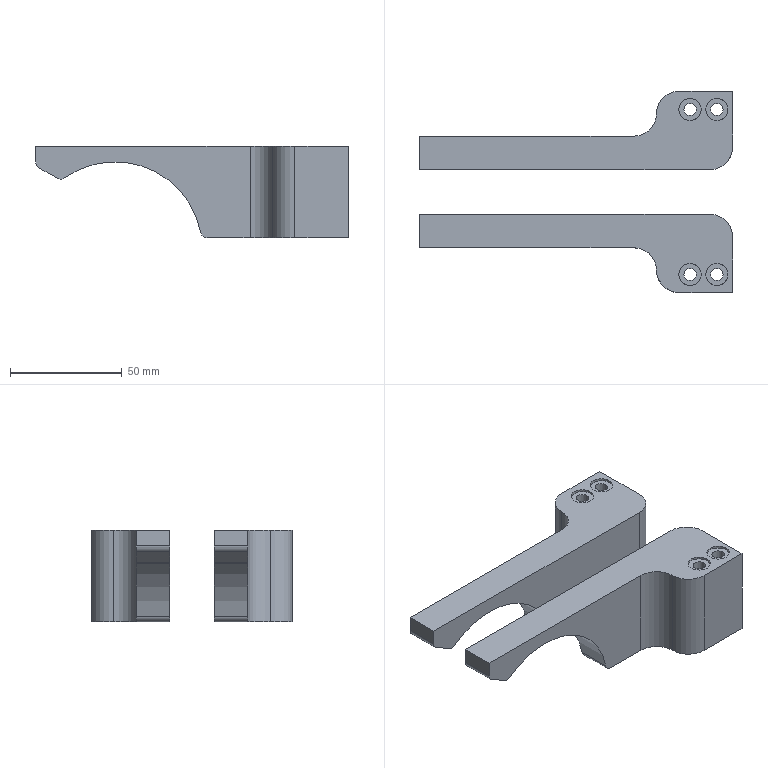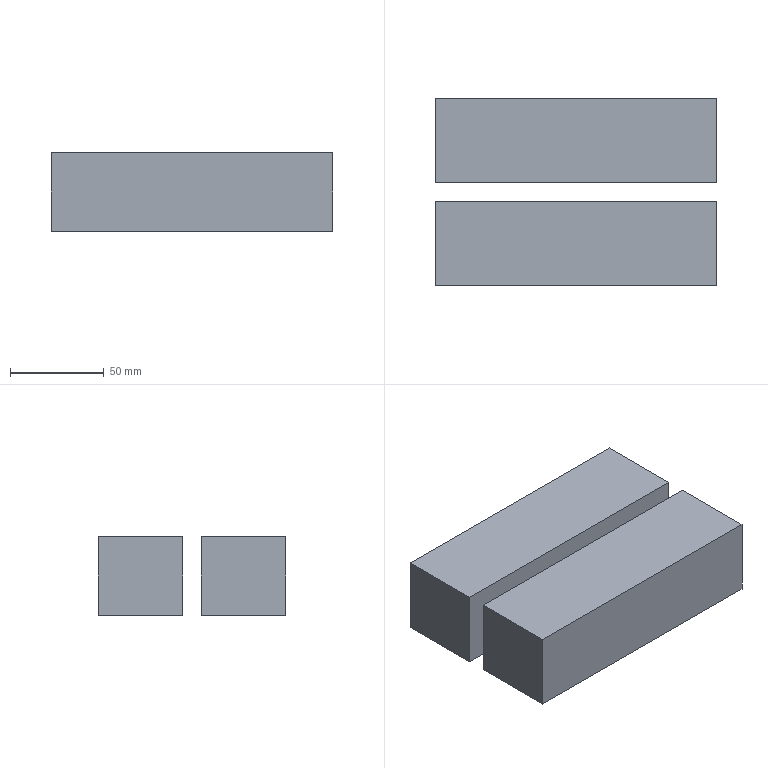CAM job | NX | 3-axis milling, drilling | part box 140 x 90 x 41 mm | stock box 150 x 100 x 42 mm
Tools:
number,name,description,diameter,corner_radius,flute_length,length,flutes
1,D63,Milling Tool-5 Parameters,63.0,0.0,50.0,75.0,2
7,D6A45,Milling Tool-5 Parameters,6.0,0.0,50.0,75.0,2
15,5.5ZT,Drilling Tool,5.5,0.0,35.0,50.0,2
12,D12C,Milling Tool-5 Parameters,12.0,0.0,50.0,75.0,2
11,D12JING,Milling Tool-5 Parameters,12.0,0.0,50.0,75.0,2
8,R4,Milling Tool-5 Parameters,8.0,4.0,50.0,75.0,2
Operations:
program,operation,operation_type,tool,method,geometry_group,spindle_rpm,surface_speed,feed_per_tooth,feed_cut,feed_plunge,cut_length_mm,path_length_mm,cut_time_min,machine_time_min
1,FLOOR_WALL,VolumeBased25DMillingOperation,D63,METHOD,A,6500.0,1286.0,0.1154,1500.0,100.0,225.0,279.0,0.15,0.1554
1,DRILLING,Operation,D6A45,METHOD,A,5000.0,94.0,0.025,250.0,0.0,8.0,91.369,0.032,0.0403
1,DRILLING_COPY,Operation,5.5ZT,METHOD,A,2000.0,34.0,0.05,200.0,0.0,91.305,257.979,0.4565,0.4732
1,ADAPTIVE_MILLING,CavityMilling,D12C,METHOD,A,9500.0,358.0,0.1579,3000.0,1000.0,10261.335,10497.39,3.424,3.448
1,CAVITY_MILL,CavityMilling,D12C,METHOD,A,9500.0,358.0,0.1316,2500.0,1000.0,9865.088,10397.203,4.392,4.445
1,ZLEVEL_PROFILE_COPY_COPY_COPY_1_COPY_COPY_COPY,ZLevelMilling,D12JING,METHOD,A,9500.0,358.0,0.0632,1200.0,1000.0,1152.162,1296.248,0.9624,0.9768
1,ZLEVEL_PROFILE,ZLevelMilling,D12JING,METHOD,A,9500.0,179.0,0.0868,1650.0,100.0,1027.855,1107.943,0.6229,0.631
1,PLANAR_MILL,PlanarMilling,D6A45,METHOD,A,9500.0,179.0,0.0658,1250.0,100.0,229.858,289.858,0.1839,0.1899
1,FIXED_CONTOUR,SurfaceContour,R4,METHOD,A,9500.0,119.0,0.1579,3000.0,100.0,18137.524,18223.924,6.046,6.054
2,FLOOR_WALL_COPY,VolumeBased25DMillingOperation,D63,METHOD,B,6500.0,1286.0,0.1154,1500.0,100.0,225.0,279.0,0.15,0.1554
2,DRILLING_COPY_1,Operation,D6A45,METHOD,B,5000.0,94.0,0.025,250.0,0.0,8.0,91.369,0.032,0.0403
2,DRILLING_COPY_COPY,Operation,5.5ZT,METHOD,B,2000.0,34.0,0.05,200.0,0.0,91.305,257.979,0.4565,0.4732
2,ADAPTIVE_MILLING_COPY,CavityMilling,D12C,METHOD,B,9500.0,358.0,0.1579,3000.0,1000.0,10673.706,11010.755,3.562,3.596
2,CAVITY_MILL_COPY,CavityMilling,D12C,METHOD,B,9500.0,358.0,0.1316,2500.0,1000.0,9865.291,10395.533,4.392,4.445
2,ZLEVEL_PROFILE_COPY_COPY_COPY_1_COPY_COPY_COPY_COPY,ZLevelMilling,D12JING,METHOD,B,9500.0,358.0,0.0632,1200.0,1000.0,1151.581,1295.601,0.9618,0.9762
2,ZLEVEL_PROFILE_COPY,ZLevelMilling,D12JING,METHOD,B,9500.0,179.0,0.0868,1650.0,100.0,1142.084,1232.484,0.6922,0.7012
2,PLANAR_MILL_COPY,PlanarMilling,D6A45,METHOD,B,9500.0,179.0,0.0658,1250.0,100.0,229.858,289.858,0.1839,0.1899
2,FIXED_CONTOUR_COPY,SurfaceContour,R4,METHOD,B,9500.0,119.0,0.1579,3000.0,100.0,18137.523,18223.923,6.046,6.054